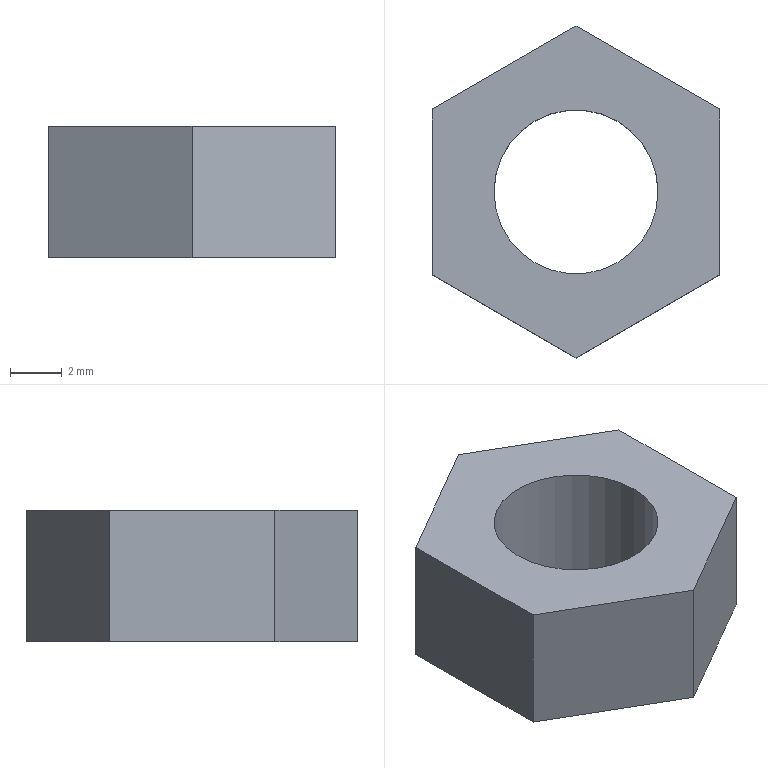Part | NX | features solid 2 | 1 solid | 9 faces | box 11.125 x 12.846 x 5.08 mm | volume 383.636 mm3 | plane 8 | cylinder 1 | commonest cylinder face diameters 6.35 x1
STEP:
#1=CARTESIAN_POINT('',(5.563,-3.212,0.));
#2=VERTEX_POINT('',#1);
#3=CARTESIAN_POINT('',(0.,-6.423,0.));
#4=VERTEX_POINT('',#3);
#5=CARTESIAN_POINT('',(5.563,-3.212,0.));
#6=DIRECTION('',(-0.866,-0.5,0.));
#7=VECTOR('',#6,1000.);
#8=LINE('',#5,#7);
#9=EDGE_CURVE('',#2,#4,#8,.T.);
#10=ORIENTED_EDGE('',*,*,#9,.F.);
#11=CARTESIAN_POINT('',(5.563,-3.212,5.08));
#12=VERTEX_POINT('',#11);
#13=CARTESIAN_POINT('',(5.563,-3.212,5.08));
#14=DIRECTION('',(0.,0.,-1.));
#15=VECTOR('',#14,1000.);
#16=LINE('',#13,#15);
#17=EDGE_CURVE('',#12,#2,#16,.T.);
#18=ORIENTED_EDGE('',*,*,#17,.F.);
#19=CARTESIAN_POINT('',(0.,-6.423,5.08));
#20=VERTEX_POINT('',#19);
#21=CARTESIAN_POINT('',(5.563,-3.212,5.08));
#22=DIRECTION('',(-0.866,-0.5,0.));
#23=VECTOR('',#22,1000.);
#24=LINE('',#21,#23);
#25=EDGE_CURVE('',#12,#20,#24,.T.);
#26=ORIENTED_EDGE('',*,*,#25,.T.);
#27=CARTESIAN_POINT('',(0.,-6.423,5.08));
#28=DIRECTION('',(0.,0.,-1.));
#29=VECTOR('',#28,1000.);
#30=LINE('',#27,#29);
#31=EDGE_CURVE('',#20,#4,#30,.T.);
#32=ORIENTED_EDGE('',*,*,#31,.T.);
#33=EDGE_LOOP('',(#10,#18,#26,#32));
#34=FACE_BOUND('',#33,.T.);
#35=CARTESIAN_POINT('',(5.563,-3.212,5.08));
#36=DIRECTION('',(0.5,-0.866,0.));
#37=DIRECTION('',(0.866,0.5,0.));
#38=AXIS2_PLACEMENT_3D('',#35,#36,#37);
#39=PLANE('',#38);
#40=ADVANCED_FACE('',(#34),#39,.T.);
#41=CARTESIAN_POINT('',(-5.563,-3.212,0.));
#42=VERTEX_POINT('',#41);
#43=CARTESIAN_POINT('',(0.,-6.423,0.));
#44=DIRECTION('',(-0.866,0.5,0.));
#45=VECTOR('',#44,1000.);
#46=LINE('',#43,#45);
#47=EDGE_CURVE('',#4,#42,#46,.T.);
#48=ORIENTED_EDGE('',*,*,#47,.F.);
#49=ORIENTED_EDGE('',*,*,#31,.F.);
#50=CARTESIAN_POINT('',(-5.563,-3.212,5.08));
#51=VERTEX_POINT('',#50);
#52=CARTESIAN_POINT('',(0.,-6.423,5.08));
#53=DIRECTION('',(-0.866,0.5,0.));
#54=VECTOR('',#53,1000.);
#55=LINE('',#52,#54);
#56=EDGE_CURVE('',#20,#51,#55,.T.);
#57=ORIENTED_EDGE('',*,*,#56,.T.);
#58=CARTESIAN_POINT('',(-5.563,-3.212,5.08));
#59=DIRECTION('',(0.,0.,-1.));
#60=VECTOR('',#59,1000.);
#61=LINE('',#58,#60);
#62=EDGE_CURVE('',#51,#42,#61,.T.);
#63=ORIENTED_EDGE('',*,*,#62,.T.);
#64=EDGE_LOOP('',(#48,#49,#57,#63));
#65=FACE_BOUND('',#64,.T.);
#66=CARTESIAN_POINT('',(0.,-6.423,5.08));
#67=DIRECTION('',(-0.5,-0.866,0.));
#68=DIRECTION('',(0.866,-0.5,0.));
#69=AXIS2_PLACEMENT_3D('',#66,#67,#68);
#70=PLANE('',#69);
#71=ADVANCED_FACE('',(#65),#70,.T.);
#72=CARTESIAN_POINT('',(-5.563,3.212,0.));
#73=VERTEX_POINT('',#72);
#74=CARTESIAN_POINT('',(-5.563,-3.212,0.));
#75=DIRECTION('',(0.,1.,0.));
#76=VECTOR('',#75,1000.);
#77=LINE('',#74,#76);
#78=EDGE_CURVE('',#42,#73,#77,.T.);
#79=ORIENTED_EDGE('',*,*,#78,.F.);
#80=ORIENTED_EDGE('',*,*,#62,.F.);
#81=CARTESIAN_POINT('',(-5.563,3.212,5.08));
#82=VERTEX_POINT('',#81);
#83=CARTESIAN_POINT('',(-5.563,-3.212,5.08));
#84=DIRECTION('',(0.,1.,0.));
#85=VECTOR('',#84,1000.);
#86=LINE('',#83,#85);
#87=EDGE_CURVE('',#51,#82,#86,.T.);
#88=ORIENTED_EDGE('',*,*,#87,.T.);
#89=CARTESIAN_POINT('',(-5.563,3.212,5.08));
#90=DIRECTION('',(0.,0.,-1.));
#91=VECTOR('',#90,1000.);
#92=LINE('',#89,#91);
#93=EDGE_CURVE('',#82,#73,#92,.T.);
#94=ORIENTED_EDGE('',*,*,#93,.T.);
#95=EDGE_LOOP('',(#79,#80,#88,#94));
#96=FACE_BOUND('',#95,.T.);
#97=CARTESIAN_POINT('',(-5.563,-3.212,5.08));
#98=DIRECTION('',(-1.,0.,0.));
#99=DIRECTION('',(0.,-1.,0.));
#100=AXIS2_PLACEMENT_3D('',#97,#98,#99);
#101=PLANE('',#100);
#102=ADVANCED_FACE('',(#96),#101,.T.);
#103=CARTESIAN_POINT('',(0.,6.423,0.));
#104=VERTEX_POINT('',#103);
#105=CARTESIAN_POINT('',(-5.563,3.212,0.));
#106=DIRECTION('',(0.866,0.5,0.));
#107=VECTOR('',#106,1000.);
#108=LINE('',#105,#107);
#109=EDGE_CURVE('',#73,#104,#108,.T.);
#110=ORIENTED_EDGE('',*,*,#109,.F.);
#111=ORIENTED_EDGE('',*,*,#93,.F.);
#112=CARTESIAN_POINT('',(0.,6.423,5.08));
#113=VERTEX_POINT('',#112);
#114=CARTESIAN_POINT('',(-5.563,3.212,5.08));
#115=DIRECTION('',(0.866,0.5,0.));
#116=VECTOR('',#115,1000.);
#117=LINE('',#114,#116);
#118=EDGE_CURVE('',#82,#113,#117,.T.);
#119=ORIENTED_EDGE('',*,*,#118,.T.);
#120=CARTESIAN_POINT('',(0.,6.423,5.08));
#121=DIRECTION('',(0.,0.,-1.));
#122=VECTOR('',#121,1000.);
#123=LINE('',#120,#122);
#124=EDGE_CURVE('',#113,#104,#123,.T.);
#125=ORIENTED_EDGE('',*,*,#124,.T.);
#126=EDGE_LOOP('',(#110,#111,#119,#125));
#127=FACE_BOUND('',#126,.T.);
#128=CARTESIAN_POINT('',(-5.563,3.212,5.08));
#129=DIRECTION('',(-0.5,0.866,0.));
#130=DIRECTION('',(-0.866,-0.5,0.));
#131=AXIS2_PLACEMENT_3D('',#128,#129,#130);
#132=PLANE('',#131);
#133=ADVANCED_FACE('',(#127),#132,.T.);
#134=CARTESIAN_POINT('',(5.563,3.212,0.));
#135=VERTEX_POINT('',#134);
#136=CARTESIAN_POINT('',(0.,6.423,0.));
#137=DIRECTION('',(0.866,-0.5,0.));
#138=VECTOR('',#137,1000.);
#139=LINE('',#136,#138);
#140=EDGE_CURVE('',#104,#135,#139,.T.);
#141=ORIENTED_EDGE('',*,*,#140,.F.);
#142=ORIENTED_EDGE('',*,*,#124,.F.);
#143=CARTESIAN_POINT('',(5.563,3.212,5.08));
#144=VERTEX_POINT('',#143);
#145=CARTESIAN_POINT('',(0.,6.423,5.08));
#146=DIRECTION('',(0.866,-0.5,0.));
#147=VECTOR('',#146,1000.);
#148=LINE('',#145,#147);
#149=EDGE_CURVE('',#113,#144,#148,.T.);
#150=ORIENTED_EDGE('',*,*,#149,.T.);
#151=CARTESIAN_POINT('',(5.563,3.212,5.08));
#152=DIRECTION('',(0.,0.,-1.));
#153=VECTOR('',#152,1000.);
#154=LINE('',#151,#153);
#155=EDGE_CURVE('',#144,#135,#154,.T.);
#156=ORIENTED_EDGE('',*,*,#155,.T.);
#157=EDGE_LOOP('',(#141,#142,#150,#156));
#158=FACE_BOUND('',#157,.T.);
#159=CARTESIAN_POINT('',(0.,6.423,5.08));
#160=DIRECTION('',(0.5,0.866,0.));
#161=DIRECTION('',(-0.866,0.5,0.));
#162=AXIS2_PLACEMENT_3D('',#159,#160,#161);
#163=PLANE('',#162);
#164=ADVANCED_FACE('',(#158),#163,.T.);
#165=CARTESIAN_POINT('',(5.563,3.212,0.));
#166=DIRECTION('',(0.,-1.,0.));
#167=VECTOR('',#166,1000.);
#168=LINE('',#165,#167);
#169=EDGE_CURVE('',#135,#2,#168,.T.);
#170=ORIENTED_EDGE('',*,*,#169,.F.);
#171=ORIENTED_EDGE('',*,*,#155,.F.);
#172=CARTESIAN_POINT('',(5.563,3.212,5.08));
#173=DIRECTION('',(0.,-1.,0.));
#174=VECTOR('',#173,1000.);
#175=LINE('',#172,#174);
#176=EDGE_CURVE('',#144,#12,#175,.T.);
#177=ORIENTED_EDGE('',*,*,#176,.T.);
#178=ORIENTED_EDGE('',*,*,#17,.T.);
#179=EDGE_LOOP('',(#170,#171,#177,#178));
#180=FACE_BOUND('',#179,.T.);
#181=CARTESIAN_POINT('',(5.563,3.212,5.08));
#182=DIRECTION('',(1.,0.,0.));
#183=DIRECTION('',(0.,1.,0.));
#184=AXIS2_PLACEMENT_3D('',#181,#182,#183);
#185=PLANE('',#184);
#186=ADVANCED_FACE('',(#180),#185,.T.);
#187=CARTESIAN_POINT('',(3.175,0.,5.08));
#188=VERTEX_POINT('',#187);
#189=CARTESIAN_POINT('',(0.,0.,5.08));
#190=DIRECTION('',(0.,0.,1.));
#191=DIRECTION('',(1.,0.,0.));
#192=AXIS2_PLACEMENT_3D('',#189,#190,#191);
#193=CIRCLE('',#192,3.175);
#194=EDGE_CURVE('',#188,#188,#193,.T.);
#195=ORIENTED_EDGE('',*,*,#194,.T.);
#196=EDGE_LOOP('',(#195));
#197=FACE_BOUND('',#196,.T.);
#198=CARTESIAN_POINT('',(3.175,0.,0.));
#199=VERTEX_POINT('',#198);
#200=CARTESIAN_POINT('',(0.,0.,0.));
#201=DIRECTION('',(0.,0.,1.));
#202=DIRECTION('',(1.,0.,0.));
#203=AXIS2_PLACEMENT_3D('',#200,#201,#202);
#204=CIRCLE('',#203,3.175);
#205=EDGE_CURVE('',#199,#199,#204,.T.);
#206=ORIENTED_EDGE('',*,*,#205,.F.);
#207=EDGE_LOOP('',(#206));
#208=FACE_BOUND('',#207,.T.);
#209=CARTESIAN_POINT('',(0.,0.,5.08));
#210=DIRECTION('',(0.,0.,-1.));
#211=DIRECTION('',(-1.,0.,0.));
#212=AXIS2_PLACEMENT_3D('',#209,#210,#211);
#213=CYLINDRICAL_SURFACE('',#212,3.175);
#214=ADVANCED_FACE('',(#197,#208),#213,.F.);
#215=ORIENTED_EDGE('',*,*,#25,.F.);
#216=ORIENTED_EDGE('',*,*,#176,.F.);
#217=ORIENTED_EDGE('',*,*,#149,.F.);
#218=ORIENTED_EDGE('',*,*,#118,.F.);
#219=ORIENTED_EDGE('',*,*,#87,.F.);
#220=ORIENTED_EDGE('',*,*,#56,.F.);
#221=EDGE_LOOP('',(#215,#216,#217,#218,#219,#220));
#222=FACE_BOUND('',#221,.T.);
#223=ORIENTED_EDGE('',*,*,#194,.F.);
#224=EDGE_LOOP('',(#223));
#225=FACE_BOUND('',#224,.T.);
#226=CARTESIAN_POINT('',(0.,0.,5.08));
#227=DIRECTION('',(0.,0.,1.));
#228=DIRECTION('',(1.,0.,0.));
#229=AXIS2_PLACEMENT_3D('',#226,#227,#228);
#230=PLANE('',#229);
#231=ADVANCED_FACE('',(#222,#225),#230,.T.);
#232=ORIENTED_EDGE('',*,*,#9,.T.);
#233=ORIENTED_EDGE('',*,*,#47,.T.);
#234=ORIENTED_EDGE('',*,*,#78,.T.);
#235=ORIENTED_EDGE('',*,*,#109,.T.);
#236=ORIENTED_EDGE('',*,*,#140,.T.);
#237=ORIENTED_EDGE('',*,*,#169,.T.);
#238=EDGE_LOOP('',(#232,#233,#234,#235,#236,#237));
#239=FACE_BOUND('',#238,.T.);
#240=ORIENTED_EDGE('',*,*,#205,.T.);
#241=EDGE_LOOP('',(#240));
#242=FACE_BOUND('',#241,.T.);
#243=CARTESIAN_POINT('',(0.,0.,0.));
#244=DIRECTION('',(0.,0.,1.));
#245=DIRECTION('',(1.,0.,0.));
#246=AXIS2_PLACEMENT_3D('',#243,#244,#245);
#247=PLANE('',#246);
#248=ADVANCED_FACE('',(#239,#242),#247,.F.);
#249=CLOSED_SHELL('',(#40,#71,#102,#133,#164,#186,#214,#231,#248));
#250=MANIFOLD_SOLID_BREP('',#249);
#251=(LENGTH_UNIT()NAMED_UNIT(*)SI_UNIT(.MILLI.,.METRE.));
#252=UNCERTAINTY_MEASURE_WITH_UNIT(LENGTH_MEASURE(0.00001),#251,'','');
#253=(NAMED_UNIT(*)PLANE_ANGLE_UNIT()SI_UNIT($,.RADIAN.));
#254=(NAMED_UNIT(*)SI_UNIT($,.STERADIAN.)SOLID_ANGLE_UNIT());
#255=(GEOMETRIC_REPRESENTATION_CONTEXT(3)GLOBAL_UNCERTAINTY_ASSIGNED_CONTEXT((#252))GLOBAL_UNIT_ASSIGNED_CONTEXT((#251,#253,#254))REPRESENTATION_CONTEXT('',''));
#256=ADVANCED_BREP_SHAPE_REPRESENTATION('',(#250),#255);